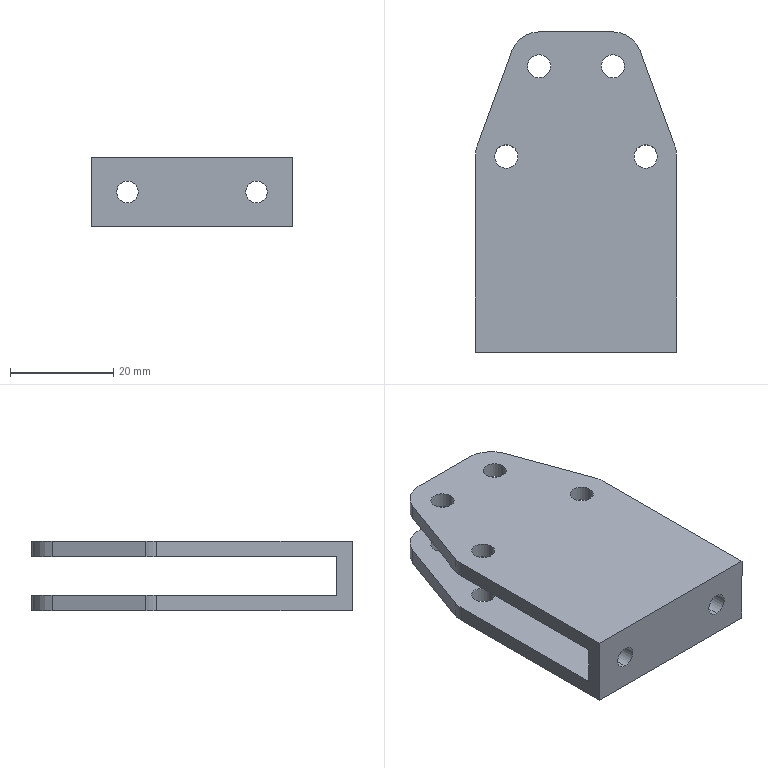Part | SolidWorks | features HoleWzd 5, ICE 5, Fillet 2, Extrusion 1, Scale 1 | 1 solid | 67 faces | box 39 x 62.088 x 13.5 mm | volume 13319 mm3 | cylinder 43 | plane 24 | commonest cylinder face diameters 4.5 x18 3 x9 12 x8 2.05 x4 4.2 x4